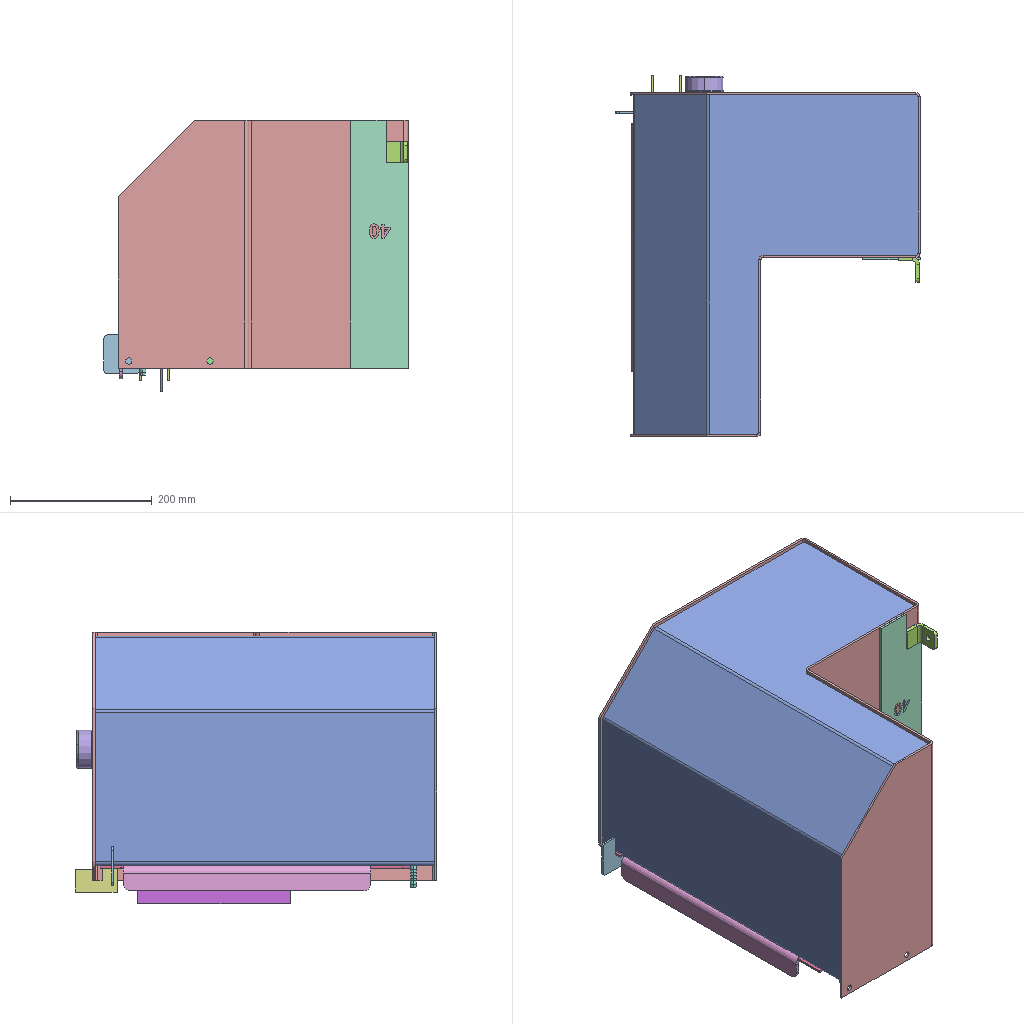Assembly | SolidWorks | 11 different items | 12 placed | box 430 x 511 x 383 mm
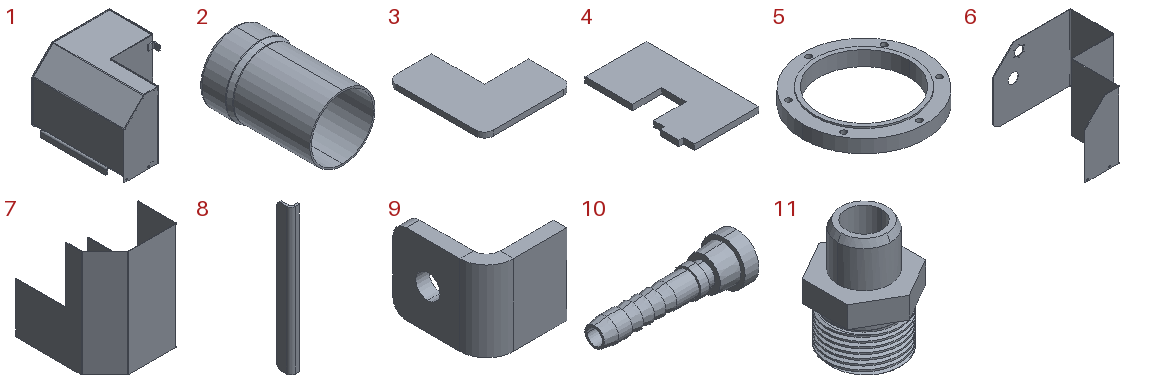Parts list (item | name | quantity | parent item | size | volume | features):
1 | (subassembly) | x1 | - | 410 x 509 x 365 mm | 2578736 mm3 | features CompositeCurve 2
2 | - | x1 | in 1 | 54.2 x 85.2 x 54.2 mm | 19561 mm3 | features BaseBody 1
3 | - | x1 | - | 50 x 55 x 3 mm | 5952 mm3 | features Extrusion 1
4 | - | x2 | - | 36.242 x 59.193 x 3 mm | 5296 mm3 | features Extrusion 1
5 | - | x1 | - | 150 x 150 x 18 mm | 130969 mm3 | features Extrusion 1, ICE 1
6 | - | x1 | in 1 | 410 x 486 x 350 mm | 1308864 mm3 | features BaseBody 1
7 | - | x1 | in 1 | 325 x 402 x 480 mm | 1150314 mm3 | features EdgeFlange 3, FlatPattern 1, SMBaseFlange 1, SheetMetal 1
8 | - | x1 | in 1 | 20 x 35 x 350 mm | 81652 mm3 | features BaseBody 1, FlatPattern 1, SheetMetal 1, SolidToSheetMetal 1
9 | - | x1 | in 1 | 30 x 35 x 30 mm | 8145 mm3 | features BaseBody 1, FlatPattern 1, SheetMetal 1, SolidToSheetMetal 1
10 | - | x1 | in 1 | 51.5 x 16 x 16 mm | 2788 mm3 | features BaseBody 1
11 | - | x1 | in 1 | 23.6 x 27.251 x 33 mm | 7269 mm3 | features BaseBody 1
Mates (type | each side: item.copy, entity, surface, feature):
In the top assembly
Concentric | assembly edge | 5.1 edge | 2 times
Concentric | 7.1 edge | 5.1 edge
Coincident | 3.1 face plane Boss-Extrude1 | 4.1 face plane Boss-Extrude1
In subassembly 1
DistanceDim | 2.1 face plane Input1 | 6.1 face plane Input1
Concentric | 6.1 edge | 2.1 edge